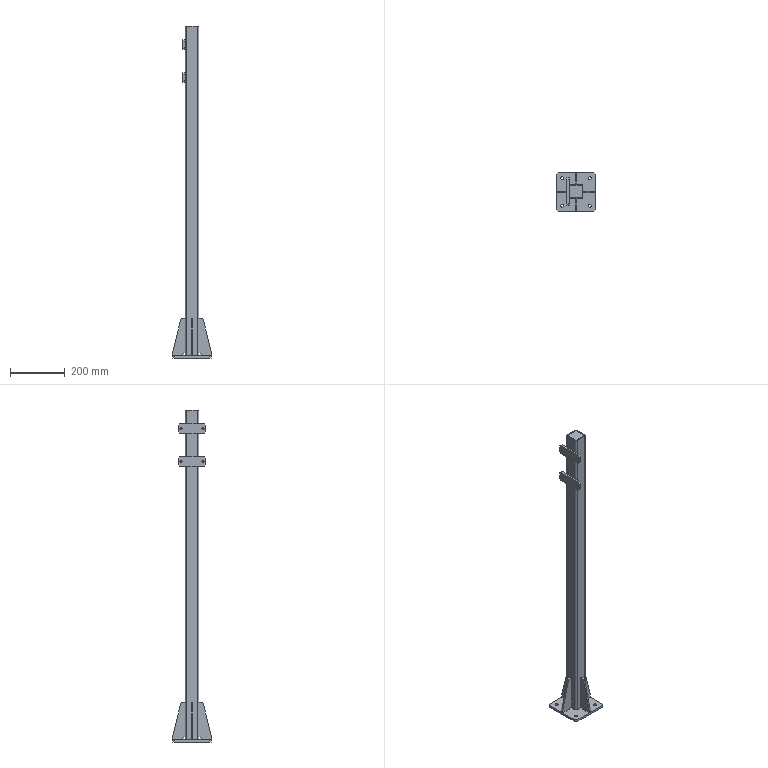Part | STEP file | HXGR200008-05-20-01 | 9 solids | 114 faces | box 140 x 140 x 1208 mm | volume 946089 mm3 | plane 78 | cylinder 28 | cone 8 | commonest cylinder face diameters 6 x8 6.8 x8 11 x8 12 x4